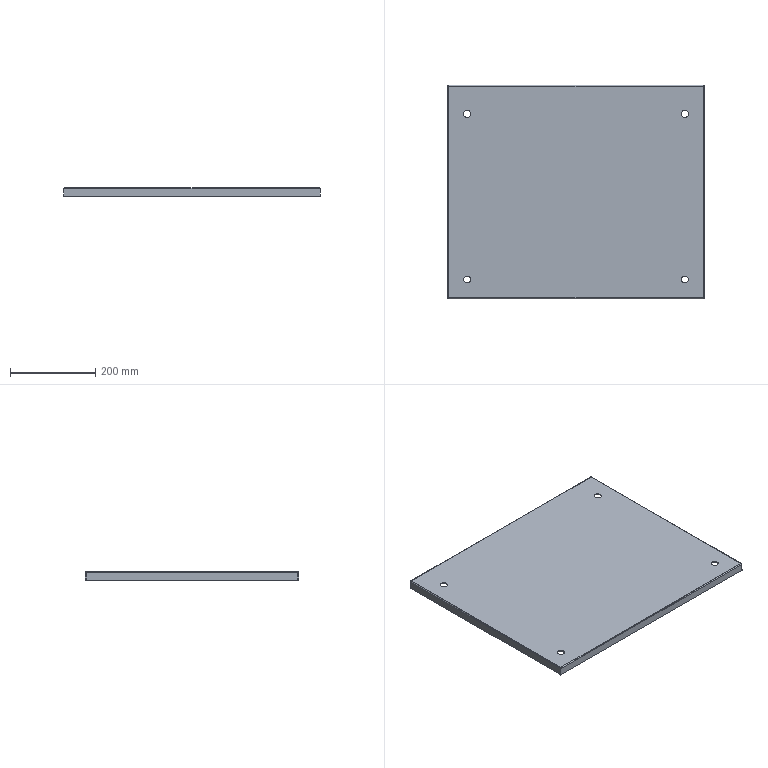Part | SolidWorks | features BaseBody 1, MoveFace 1 | 1 solid | 46 faces | box 600 x 500 x 20 mm | volume 675087 mm3 | plane 30 | cylinder 16 | commonest cylinder face diameters 0.2 x4 4.2 x4 16 x4 17 x4
STEP:
#1=CARTESIAN_POINT('',(187.,-205.,-2.));
#2=VERTEX_POINT('',#1);
#3=CARTESIAN_POINT('',(203.,-205.,-2.));
#4=VERTEX_POINT('',#3);
#5=CARTESIAN_POINT('',(195.,-205.,-2.));
#6=DIRECTION('',(0.,0.,1.));
#7=DIRECTION('',(1.,0.,0.));
#8=AXIS2_PLACEMENT_3D('',#5,#6,#7);
#9=CIRCLE('',#8,8.);
#10=EDGE_CURVE('',#2,#4,#9,.T.);
#11=ORIENTED_EDGE('',*,*,#10,.F.);
#12=CARTESIAN_POINT('',(187.,-205.,0.));
#13=VERTEX_POINT('',#12);
#14=CARTESIAN_POINT('',(187.,-205.,-10.));
#15=DIRECTION('',(0.,0.,1.));
#16=VECTOR('',#15,1000.);
#17=LINE('',#14,#16);
#18=EDGE_CURVE('',#2,#13,#17,.T.);
#19=ORIENTED_EDGE('',*,*,#18,.T.);
#20=CARTESIAN_POINT('',(203.,-205.,0.));
#21=VERTEX_POINT('',#20);
#22=CARTESIAN_POINT('',(195.,-205.,0.));
#23=DIRECTION('',(0.,0.,-1.));
#24=DIRECTION('',(1.,0.,0.));
#25=AXIS2_PLACEMENT_3D('',#22,#23,#24);
#26=CIRCLE('',#25,8.);
#27=EDGE_CURVE('',#21,#13,#26,.T.);
#28=ORIENTED_EDGE('',*,*,#27,.F.);
#29=CARTESIAN_POINT('',(203.,-205.,-10.));
#30=DIRECTION('',(0.,0.,1.));
#31=VECTOR('',#30,1000.);
#32=LINE('',#29,#31);
#33=EDGE_CURVE('',#4,#21,#32,.T.);
#34=ORIENTED_EDGE('',*,*,#33,.F.);
#35=EDGE_LOOP('',(#11,#19,#28,#34));
#36=FACE_OUTER_BOUND('',#35,.T.);
#37=CARTESIAN_POINT('',(195.,-205.,-10.));
#38=DIRECTION('',(0.,0.,1.));
#39=DIRECTION('',(1.,0.,0.));
#40=AXIS2_PLACEMENT_3D('',#37,#38,#39);
#41=CYLINDRICAL_SURFACE('',#40,8.);
#42=ADVANCED_FACE('',(#36),#41,.F.);
#43=CARTESIAN_POINT('',(-323.,-205.,-2.));
#44=VERTEX_POINT('',#43);
#45=CARTESIAN_POINT('',(-307.,-205.,-2.));
#46=VERTEX_POINT('',#45);
#47=CARTESIAN_POINT('',(-315.,-205.,-2.));
#48=DIRECTION('',(0.,0.,1.));
#49=DIRECTION('',(1.,0.,0.));
#50=AXIS2_PLACEMENT_3D('',#47,#48,#49);
#51=CIRCLE('',#50,8.);
#52=EDGE_CURVE('',#44,#46,#51,.T.);
#53=ORIENTED_EDGE('',*,*,#52,.F.);
#54=CARTESIAN_POINT('',(-323.,-205.,0.));
#55=VERTEX_POINT('',#54);
#56=CARTESIAN_POINT('',(-323.,-205.,-10.));
#57=DIRECTION('',(0.,0.,1.));
#58=VECTOR('',#57,1000.);
#59=LINE('',#56,#58);
#60=EDGE_CURVE('',#44,#55,#59,.T.);
#61=ORIENTED_EDGE('',*,*,#60,.T.);
#62=CARTESIAN_POINT('',(-307.,-205.,0.));
#63=VERTEX_POINT('',#62);
#64=CARTESIAN_POINT('',(-315.,-205.,0.));
#65=DIRECTION('',(0.,0.,-1.));
#66=DIRECTION('',(1.,0.,0.));
#67=AXIS2_PLACEMENT_3D('',#64,#65,#66);
#68=CIRCLE('',#67,8.);
#69=EDGE_CURVE('',#63,#55,#68,.T.);
#70=ORIENTED_EDGE('',*,*,#69,.F.);
#71=CARTESIAN_POINT('',(-307.,-205.,-10.));
#72=DIRECTION('',(0.,0.,1.));
#73=VECTOR('',#72,1000.);
#74=LINE('',#71,#73);
#75=EDGE_CURVE('',#46,#63,#74,.T.);
#76=ORIENTED_EDGE('',*,*,#75,.F.);
#77=EDGE_LOOP('',(#53,#61,#70,#76));
#78=FACE_OUTER_BOUND('',#77,.T.);
#79=CARTESIAN_POINT('',(-315.,-205.,-10.));
#80=DIRECTION('',(0.,0.,1.));
#81=DIRECTION('',(1.,0.,0.));
#82=AXIS2_PLACEMENT_3D('',#79,#80,#81);
#83=CYLINDRICAL_SURFACE('',#82,8.);
#84=ADVANCED_FACE('',(#78),#83,.F.);
#85=CARTESIAN_POINT('',(-323.5,183.,-2.));
#86=VERTEX_POINT('',#85);
#87=CARTESIAN_POINT('',(-306.5,183.,-2.));
#88=VERTEX_POINT('',#87);
#89=CARTESIAN_POINT('',(-315.,183.,-2.));
#90=DIRECTION('',(0.,0.,1.));
#91=DIRECTION('',(1.,0.,0.));
#92=AXIS2_PLACEMENT_3D('',#89,#90,#91);
#93=CIRCLE('',#92,8.5);
#94=EDGE_CURVE('',#86,#88,#93,.T.);
#95=ORIENTED_EDGE('',*,*,#94,.F.);
#96=CARTESIAN_POINT('',(-323.5,183.,0.));
#97=VERTEX_POINT('',#96);
#98=CARTESIAN_POINT('',(-323.5,183.,-10.));
#99=DIRECTION('',(0.,0.,1.));
#100=VECTOR('',#99,1000.);
#101=LINE('',#98,#100);
#102=EDGE_CURVE('',#86,#97,#101,.T.);
#103=ORIENTED_EDGE('',*,*,#102,.T.);
#104=CARTESIAN_POINT('',(-306.5,183.,0.));
#105=VERTEX_POINT('',#104);
#106=CARTESIAN_POINT('',(-315.,183.,0.));
#107=DIRECTION('',(0.,0.,-1.));
#108=DIRECTION('',(1.,0.,0.));
#109=AXIS2_PLACEMENT_3D('',#106,#107,#108);
#110=CIRCLE('',#109,8.5);
#111=EDGE_CURVE('',#105,#97,#110,.T.);
#112=ORIENTED_EDGE('',*,*,#111,.F.);
#113=CARTESIAN_POINT('',(-306.5,183.,-10.));
#114=DIRECTION('',(0.,0.,1.));
#115=VECTOR('',#114,1000.);
#116=LINE('',#113,#115);
#117=EDGE_CURVE('',#88,#105,#116,.T.);
#118=ORIENTED_EDGE('',*,*,#117,.F.);
#119=EDGE_LOOP('',(#95,#103,#112,#118));
#120=FACE_OUTER_BOUND('',#119,.T.);
#121=CARTESIAN_POINT('',(-315.,183.,-10.));
#122=DIRECTION('',(0.,0.,1.));
#123=DIRECTION('',(1.,0.,0.));
#124=AXIS2_PLACEMENT_3D('',#121,#122,#123);
#125=CYLINDRICAL_SURFACE('',#124,8.5);
#126=ADVANCED_FACE('',(#120),#125,.F.);
#127=CARTESIAN_POINT('',(186.5,183.,-2.));
#128=VERTEX_POINT('',#127);
#129=CARTESIAN_POINT('',(203.5,183.,-2.));
#130=VERTEX_POINT('',#129);
#131=CARTESIAN_POINT('',(195.,183.,-2.));
#132=DIRECTION('',(0.,0.,1.));
#133=DIRECTION('',(1.,0.,0.));
#134=AXIS2_PLACEMENT_3D('',#131,#132,#133);
#135=CIRCLE('',#134,8.5);
#136=EDGE_CURVE('',#128,#130,#135,.T.);
#137=ORIENTED_EDGE('',*,*,#136,.F.);
#138=CARTESIAN_POINT('',(186.5,183.,0.));
#139=VERTEX_POINT('',#138);
#140=CARTESIAN_POINT('',(186.5,183.,-10.));
#141=DIRECTION('',(0.,0.,1.));
#142=VECTOR('',#141,1000.);
#143=LINE('',#140,#142);
#144=EDGE_CURVE('',#128,#139,#143,.T.);
#145=ORIENTED_EDGE('',*,*,#144,.T.);
#146=CARTESIAN_POINT('',(203.5,183.,0.));
#147=VERTEX_POINT('',#146);
#148=CARTESIAN_POINT('',(195.,183.,0.));
#149=DIRECTION('',(0.,0.,-1.));
#150=DIRECTION('',(1.,0.,0.));
#151=AXIS2_PLACEMENT_3D('',#148,#149,#150);
#152=CIRCLE('',#151,8.5);
#153=EDGE_CURVE('',#147,#139,#152,.T.);
#154=ORIENTED_EDGE('',*,*,#153,.F.);
#155=CARTESIAN_POINT('',(203.5,183.,-10.));
#156=DIRECTION('',(0.,0.,1.));
#157=VECTOR('',#156,1000.);
#158=LINE('',#155,#157);
#159=EDGE_CURVE('',#130,#147,#158,.T.);
#160=ORIENTED_EDGE('',*,*,#159,.F.);
#161=EDGE_LOOP('',(#137,#145,#154,#160));
#162=FACE_OUTER_BOUND('',#161,.T.);
#163=CARTESIAN_POINT('',(195.,183.,-10.));
#164=DIRECTION('',(0.,0.,1.));
#165=DIRECTION('',(1.,0.,0.));
#166=AXIS2_PLACEMENT_3D('',#163,#164,#165);
#167=CYLINDRICAL_SURFACE('',#166,8.5);
#168=ADVANCED_FACE('',(#162),#167,.F.);
#169=CARTESIAN_POINT('',(237.9,247.9,0.));
#170=VERTEX_POINT('',#169);
#171=CARTESIAN_POINT('',(-357.9,247.9,0.));
#172=VERTEX_POINT('',#171);
#173=CARTESIAN_POINT('',(0.,247.9,0.));
#174=DIRECTION('',(-1.,0.,0.));
#175=VECTOR('',#174,1000.);
#176=LINE('',#173,#175);
#177=EDGE_CURVE('',#170,#172,#176,.T.);
#178=ORIENTED_EDGE('',*,*,#177,.T.);
#179=CARTESIAN_POINT('',(-357.9,-247.9,0.));
#180=VERTEX_POINT('',#179);
#181=CARTESIAN_POINT('',(-357.9,0.,0.));
#182=DIRECTION('',(0.,-1.,0.));
#183=VECTOR('',#182,1000.);
#184=LINE('',#181,#183);
#185=EDGE_CURVE('',#172,#180,#184,.T.);
#186=ORIENTED_EDGE('',*,*,#185,.T.);
#187=CARTESIAN_POINT('',(237.9,-247.9,0.));
#188=VERTEX_POINT('',#187);
#189=CARTESIAN_POINT('',(0.,-247.9,0.));
#190=DIRECTION('',(1.,0.,0.));
#191=VECTOR('',#190,1000.);
#192=LINE('',#189,#191);
#193=EDGE_CURVE('',#180,#188,#192,.T.);
#194=ORIENTED_EDGE('',*,*,#193,.T.);
#195=CARTESIAN_POINT('',(237.9,0.,0.));
#196=DIRECTION('',(0.,1.,0.));
#197=VECTOR('',#196,1000.);
#198=LINE('',#195,#197);
#199=EDGE_CURVE('',#188,#170,#198,.T.);
#200=ORIENTED_EDGE('',*,*,#199,.T.);
#201=EDGE_LOOP('',(#178,#186,#194,#200));
#202=FACE_OUTER_BOUND('',#201,.T.);
#203=ORIENTED_EDGE('',*,*,#27,.T.);
#204=CARTESIAN_POINT('',(195.,-205.,0.));
#205=DIRECTION('',(0.,0.,-1.));
#206=DIRECTION('',(1.,0.,0.));
#207=AXIS2_PLACEMENT_3D('',#204,#205,#206);
#208=CIRCLE('',#207,8.);
#209=EDGE_CURVE('',#13,#21,#208,.T.);
#210=ORIENTED_EDGE('',*,*,#209,.T.);
#211=EDGE_LOOP('',(#203,#210));
#212=FACE_BOUND('',#211,.T.);
#213=ORIENTED_EDGE('',*,*,#69,.T.);
#214=CARTESIAN_POINT('',(-315.,-205.,0.));
#215=DIRECTION('',(0.,0.,-1.));
#216=DIRECTION('',(1.,0.,0.));
#217=AXIS2_PLACEMENT_3D('',#214,#215,#216);
#218=CIRCLE('',#217,8.);
#219=EDGE_CURVE('',#55,#63,#218,.T.);
#220=ORIENTED_EDGE('',*,*,#219,.T.);
#221=EDGE_LOOP('',(#213,#220));
#222=FACE_BOUND('',#221,.T.);
#223=ORIENTED_EDGE('',*,*,#111,.T.);
#224=CARTESIAN_POINT('',(-315.,183.,0.));
#225=DIRECTION('',(0.,0.,-1.));
#226=DIRECTION('',(1.,0.,0.));
#227=AXIS2_PLACEMENT_3D('',#224,#225,#226);
#228=CIRCLE('',#227,8.5);
#229=EDGE_CURVE('',#97,#105,#228,.T.);
#230=ORIENTED_EDGE('',*,*,#229,.T.);
#231=EDGE_LOOP('',(#223,#230));
#232=FACE_BOUND('',#231,.T.);
#233=ORIENTED_EDGE('',*,*,#153,.T.);
#234=CARTESIAN_POINT('',(195.,183.,0.));
#235=DIRECTION('',(0.,0.,-1.));
#236=DIRECTION('',(1.,0.,0.));
#237=AXIS2_PLACEMENT_3D('',#234,#235,#236);
#238=CIRCLE('',#237,8.5);
#239=EDGE_CURVE('',#139,#147,#238,.T.);
#240=ORIENTED_EDGE('',*,*,#239,.T.);
#241=EDGE_LOOP('',(#233,#240));
#242=FACE_BOUND('',#241,.T.);
#243=CARTESIAN_POINT('',(0.,0.,0.));
#244=DIRECTION('',(0.,0.,1.));
#245=DIRECTION('',(1.,0.,0.));
#246=AXIS2_PLACEMENT_3D('',#243,#244,#245);
#247=PLANE('',#246);
#248=ADVANCED_FACE('',(#202,#212,#222,#232,#242),#247,.T.);
#249=CARTESIAN_POINT('',(-360.,247.9,-2.1));
#250=VERTEX_POINT('',#249);
#251=CARTESIAN_POINT('',(-360.,-247.9,-2.1));
#252=VERTEX_POINT('',#251);
#253=CARTESIAN_POINT('',(-360.,247.9,-2.1));
#254=DIRECTION('',(0.,-1.,0.));
#255=VECTOR('',#254,1000.);
#256=LINE('',#253,#255);
#257=EDGE_CURVE('',#250,#252,#256,.T.);
#258=ORIENTED_EDGE('',*,*,#257,.T.);
#259=CARTESIAN_POINT('',(-357.9,-247.9,-2.1));
#260=DIRECTION('',(0.,1.,0.));
#261=DIRECTION('',(0.,0.,1.));
#262=AXIS2_PLACEMENT_3D('',#259,#260,#261);
#263=CIRCLE('',#262,2.1);
#264=EDGE_CURVE('',#252,#180,#263,.T.);
#265=ORIENTED_EDGE('',*,*,#264,.T.);
#266=ORIENTED_EDGE('',*,*,#185,.F.);
#267=CARTESIAN_POINT('',(-357.9,247.9,-2.1));
#268=DIRECTION('',(0.,-1.,0.));
#269=DIRECTION('',(0.,0.,1.));
#270=AXIS2_PLACEMENT_3D('',#267,#268,#269);
#271=CIRCLE('',#270,2.1);
#272=EDGE_CURVE('',#172,#250,#271,.T.);
#273=ORIENTED_EDGE('',*,*,#272,.T.);
#274=EDGE_LOOP('',(#258,#265,#266,#273));
#275=FACE_OUTER_BOUND('',#274,.T.);
#276=CARTESIAN_POINT('',(-357.9,247.9,-2.1));
#277=DIRECTION('',(0.,1.,0.));
#278=DIRECTION('',(0.,0.,1.));
#279=AXIS2_PLACEMENT_3D('',#276,#277,#278);
#280=CYLINDRICAL_SURFACE('',#279,2.1);
#281=ADVANCED_FACE('',(#275),#280,.T.);
#282=CARTESIAN_POINT('',(237.9,250.,-2.1));
#283=VERTEX_POINT('',#282);
#284=CARTESIAN_POINT('',(-357.9,250.,-2.1));
#285=VERTEX_POINT('',#284);
#286=CARTESIAN_POINT('',(360.,250.,-2.1));
#287=DIRECTION('',(-1.,0.,0.));
#288=VECTOR('',#287,1000.);
#289=LINE('',#286,#288);
#290=EDGE_CURVE('',#283,#285,#289,.T.);
#291=ORIENTED_EDGE('',*,*,#290,.T.);
#292=CARTESIAN_POINT('',(-357.9,247.9,-2.1));
#293=DIRECTION('',(1.,0.,0.));
#294=DIRECTION('',(0.,0.,-1.));
#295=AXIS2_PLACEMENT_3D('',#292,#293,#294);
#296=CIRCLE('',#295,2.1);
#297=EDGE_CURVE('',#285,#172,#296,.T.);
#298=ORIENTED_EDGE('',*,*,#297,.T.);
#299=ORIENTED_EDGE('',*,*,#177,.F.);
#300=CARTESIAN_POINT('',(237.9,247.9,-2.1));
#301=DIRECTION('',(-1.,0.,0.));
#302=DIRECTION('',(0.,0.,-1.));
#303=AXIS2_PLACEMENT_3D('',#300,#301,#302);
#304=CIRCLE('',#303,2.1);
#305=EDGE_CURVE('',#170,#283,#304,.T.);
#306=ORIENTED_EDGE('',*,*,#305,.T.);
#307=EDGE_LOOP('',(#291,#298,#299,#306));
#308=FACE_OUTER_BOUND('',#307,.T.);
#309=CARTESIAN_POINT('',(360.,247.9,-2.1));
#310=DIRECTION('',(1.,0.,0.));
#311=DIRECTION('',(0.,0.,-1.));
#312=AXIS2_PLACEMENT_3D('',#309,#310,#311);
#313=CYLINDRICAL_SURFACE('',#312,2.1);
#314=ADVANCED_FACE('',(#308),#313,.T.);
#315=CARTESIAN_POINT('',(240.,-247.9,-2.1));
#316=VERTEX_POINT('',#315);
#317=CARTESIAN_POINT('',(240.,247.9,-2.1));
#318=VERTEX_POINT('',#317);
#319=CARTESIAN_POINT('',(240.,-247.9,-2.1));
#320=DIRECTION('',(0.,1.,0.));
#321=VECTOR('',#320,1000.);
#322=LINE('',#319,#321);
#323=EDGE_CURVE('',#316,#318,#322,.T.);
#324=ORIENTED_EDGE('',*,*,#323,.T.);
#325=CARTESIAN_POINT('',(237.9,247.9,-2.1));
#326=DIRECTION('',(0.,-1.,0.));
#327=DIRECTION('',(0.,0.,-1.));
#328=AXIS2_PLACEMENT_3D('',#325,#326,#327);
#329=CIRCLE('',#328,2.1);
#330=EDGE_CURVE('',#318,#170,#329,.T.);
#331=ORIENTED_EDGE('',*,*,#330,.T.);
#332=ORIENTED_EDGE('',*,*,#199,.F.);
#333=CARTESIAN_POINT('',(237.9,-247.9,-2.1));
#334=DIRECTION('',(0.,1.,0.));
#335=DIRECTION('',(0.,0.,-1.));
#336=AXIS2_PLACEMENT_3D('',#333,#334,#335);
#337=CIRCLE('',#336,2.1);
#338=EDGE_CURVE('',#188,#316,#337,.T.);
#339=ORIENTED_EDGE('',*,*,#338,.T.);
#340=EDGE_LOOP('',(#324,#331,#332,#339));
#341=FACE_OUTER_BOUND('',#340,.T.);
#342=CARTESIAN_POINT('',(237.9,-247.9,-2.1));
#343=DIRECTION('',(0.,-1.,0.));
#344=DIRECTION('',(0.,0.,-1.));
#345=AXIS2_PLACEMENT_3D('',#342,#343,#344);
#346=CYLINDRICAL_SURFACE('',#345,2.1);
#347=ADVANCED_FACE('',(#341),#346,.T.);
#348=ORIENTED_EDGE('',*,*,#193,.F.);
#349=CARTESIAN_POINT('',(-357.9,-250.,-2.1));
#350=VERTEX_POINT('',#349);
#351=CARTESIAN_POINT('',(-357.9,-247.9,-2.1));
#352=DIRECTION('',(1.,0.,0.));
#353=DIRECTION('',(0.,0.,1.));
#354=AXIS2_PLACEMENT_3D('',#351,#352,#353);
#355=CIRCLE('',#354,2.1);
#356=EDGE_CURVE('',#180,#350,#355,.T.);
#357=ORIENTED_EDGE('',*,*,#356,.T.);
#358=CARTESIAN_POINT('',(237.9,-250.,-2.1));
#359=VERTEX_POINT('',#358);
#360=CARTESIAN_POINT('',(-360.,-250.,-2.1));
#361=DIRECTION('',(1.,0.,0.));
#362=VECTOR('',#361,1000.);
#363=LINE('',#360,#362);
#364=EDGE_CURVE('',#350,#359,#363,.T.);
#365=ORIENTED_EDGE('',*,*,#364,.T.);
#366=CARTESIAN_POINT('',(237.9,-247.9,-2.1));
#367=DIRECTION('',(-1.,0.,0.));
#368=DIRECTION('',(0.,0.,1.));
#369=AXIS2_PLACEMENT_3D('',#366,#367,#368);
#370=CIRCLE('',#369,2.1);
#371=EDGE_CURVE('',#359,#188,#370,.T.);
#372=ORIENTED_EDGE('',*,*,#371,.T.);
#373=EDGE_LOOP('',(#348,#357,#365,#372));
#374=FACE_OUTER_BOUND('',#373,.T.);
#375=CARTESIAN_POINT('',(-360.,-247.9,-2.1));
#376=DIRECTION('',(-1.,0.,0.));
#377=DIRECTION('',(0.,0.,1.));
#378=AXIS2_PLACEMENT_3D('',#375,#376,#377);
#379=CYLINDRICAL_SURFACE('',#378,2.1);
#380=ADVANCED_FACE('',(#374),#379,.T.);
#381=ORIENTED_EDGE('',*,*,#18,.F.);
#382=CARTESIAN_POINT('',(195.,-205.,-2.));
#383=DIRECTION('',(0.,0.,1.));
#384=DIRECTION('',(1.,0.,0.));
#385=AXIS2_PLACEMENT_3D('',#382,#383,#384);
#386=CIRCLE('',#385,8.);
#387=EDGE_CURVE('',#4,#2,#386,.T.);
#388=ORIENTED_EDGE('',*,*,#387,.F.);
#389=ORIENTED_EDGE('',*,*,#33,.T.);
#390=ORIENTED_EDGE('',*,*,#209,.F.);
#391=EDGE_LOOP('',(#381,#388,#389,#390));
#392=FACE_OUTER_BOUND('',#391,.T.);
#393=CARTESIAN_POINT('',(195.,-205.,-10.));
#394=DIRECTION('',(0.,0.,1.));
#395=DIRECTION('',(1.,0.,0.));
#396=AXIS2_PLACEMENT_3D('',#393,#394,#395);
#397=CYLINDRICAL_SURFACE('',#396,8.);
#398=ADVANCED_FACE('',(#392),#397,.F.);
#399=ORIENTED_EDGE('',*,*,#60,.F.);
#400=CARTESIAN_POINT('',(-315.,-205.,-2.));
#401=DIRECTION('',(0.,0.,1.));
#402=DIRECTION('',(1.,0.,0.));
#403=AXIS2_PLACEMENT_3D('',#400,#401,#402);
#404=CIRCLE('',#403,8.);
#405=EDGE_CURVE('',#46,#44,#404,.T.);
#406=ORIENTED_EDGE('',*,*,#405,.F.);
#407=ORIENTED_EDGE('',*,*,#75,.T.);
#408=ORIENTED_EDGE('',*,*,#219,.F.);
#409=EDGE_LOOP('',(#399,#406,#407,#408));
#410=FACE_OUTER_BOUND('',#409,.T.);
#411=CARTESIAN_POINT('',(-315.,-205.,-10.));
#412=DIRECTION('',(0.,0.,1.));
#413=DIRECTION('',(1.,0.,0.));
#414=AXIS2_PLACEMENT_3D('',#411,#412,#413);
#415=CYLINDRICAL_SURFACE('',#414,8.);
#416=ADVANCED_FACE('',(#410),#415,.F.);
#417=ORIENTED_EDGE('',*,*,#102,.F.);
#418=CARTESIAN_POINT('',(-315.,183.,-2.));
#419=DIRECTION('',(0.,0.,1.));
#420=DIRECTION('',(1.,0.,0.));
#421=AXIS2_PLACEMENT_3D('',#418,#419,#420);
#422=CIRCLE('',#421,8.5);
#423=EDGE_CURVE('',#88,#86,#422,.T.);
#424=ORIENTED_EDGE('',*,*,#423,.F.);
#425=ORIENTED_EDGE('',*,*,#117,.T.);
#426=ORIENTED_EDGE('',*,*,#229,.F.);
#427=EDGE_LOOP('',(#417,#424,#425,#426));
#428=FACE_OUTER_BOUND('',#427,.T.);
#429=CARTESIAN_POINT('',(-315.,183.,-10.));
#430=DIRECTION('',(0.,0.,1.));
#431=DIRECTION('',(1.,0.,0.));
#432=AXIS2_PLACEMENT_3D('',#429,#430,#431);
#433=CYLINDRICAL_SURFACE('',#432,8.5);
#434=ADVANCED_FACE('',(#428),#433,.F.);
#435=ORIENTED_EDGE('',*,*,#144,.F.);
#436=CARTESIAN_POINT('',(195.,183.,-2.));
#437=DIRECTION('',(0.,0.,1.));
#438=DIRECTION('',(1.,0.,0.));
#439=AXIS2_PLACEMENT_3D('',#436,#437,#438);
#440=CIRCLE('',#439,8.5);
#441=EDGE_CURVE('',#130,#128,#440,.T.);
#442=ORIENTED_EDGE('',*,*,#441,.F.);
#443=ORIENTED_EDGE('',*,*,#159,.T.);
#444=ORIENTED_EDGE('',*,*,#239,.F.);
#445=EDGE_LOOP('',(#435,#442,#443,#444));
#446=FACE_OUTER_BOUND('',#445,.T.);
#447=CARTESIAN_POINT('',(195.,183.,-10.));
#448=DIRECTION('',(0.,0.,1.));
#449=DIRECTION('',(1.,0.,0.));
#450=AXIS2_PLACEMENT_3D('',#447,#448,#449);
#451=CYLINDRICAL_SURFACE('',#450,8.5);
#452=ADVANCED_FACE('',(#446),#451,.F.);
#453=CARTESIAN_POINT('',(-357.9,-247.9,-2.));
#454=VERTEX_POINT('',#453);
#455=CARTESIAN_POINT('',(-357.9,-247.9,-2.1));
#456=DIRECTION('',(0.,0.,1.));
#457=VECTOR('',#456,1000.);
#458=LINE('',#455,#457);
#459=EDGE_CURVE('',#454,#180,#458,.T.);
#460=ORIENTED_EDGE('',*,*,#459,.T.);
#461=ORIENTED_EDGE('',*,*,#264,.F.);
#462=CARTESIAN_POINT('',(-360.,-247.9,-20.));
#463=VERTEX_POINT('',#462);
#464=CARTESIAN_POINT('',(-360.,-247.9,0.));
#465=DIRECTION('',(0.,0.,-1.));
#466=VECTOR('',#465,1000.);
#467=LINE('',#464,#466);
#468=EDGE_CURVE('',#252,#463,#467,.T.);
#469=ORIENTED_EDGE('',*,*,#468,.T.);
#470=CARTESIAN_POINT('',(-358.,-247.9,-20.));
#471=VERTEX_POINT('',#470);
#472=CARTESIAN_POINT('',(-360.,-247.9,-20.));
#473=DIRECTION('',(-1.,0.,0.));
#474=VECTOR('',#473,1000.);
#475=LINE('',#472,#474);
#476=EDGE_CURVE('',#471,#463,#475,.T.);
#477=ORIENTED_EDGE('',*,*,#476,.F.);
#478=CARTESIAN_POINT('',(-358.,-247.9,-2.1));
#479=VERTEX_POINT('',#478);
#480=CARTESIAN_POINT('',(-358.,-247.9,-2.));
#481=DIRECTION('',(0.,0.,-1.));
#482=VECTOR('',#481,1000.);
#483=LINE('',#480,#482);
#484=EDGE_CURVE('',#479,#471,#483,.T.);
#485=ORIENTED_EDGE('',*,*,#484,.F.);
#486=CARTESIAN_POINT('',(-357.9,-247.9,-2.1));
#487=DIRECTION('',(0.,1.,0.));
#488=DIRECTION('',(0.,0.,1.));
#489=AXIS2_PLACEMENT_3D('',#486,#487,#488);
#490=CIRCLE('',#489,0.1);
#491=EDGE_CURVE('',#479,#454,#490,.T.);
#492=ORIENTED_EDGE('',*,*,#491,.T.);
#493=EDGE_LOOP('',(#460,#461,#469,#477,#485,#492));
#494=FACE_OUTER_BOUND('',#493,.T.);
#495=CARTESIAN_POINT('',(-357.9,-247.9,-2.1));
#496=DIRECTION('',(0.,-1.,0.));
#497=DIRECTION('',(0.,0.,-1.));
#498=AXIS2_PLACEMENT_3D('',#495,#496,#497);
#499=PLANE('',#498);
#500=ADVANCED_FACE('',(#494),#499,.T.);
#501=CARTESIAN_POINT('',(-360.,247.9,-20.));
#502=VERTEX_POINT('',#501);
#503=CARTESIAN_POINT('',(-360.,247.9,0.));
#504=DIRECTION('',(0.,0.,1.));
#505=VECTOR('',#504,1000.);
#506=LINE('',#503,#505);
#507=EDGE_CURVE('',#502,#250,#506,.T.);
#508=ORIENTED_EDGE('',*,*,#507,.F.);
#509=CARTESIAN_POINT('',(-360.,0.,-20.));
#510=DIRECTION('',(0.,1.,0.));
#511=VECTOR('',#510,1000.);
#512=LINE('',#509,#511);
#513=EDGE_CURVE('',#463,#502,#512,.T.);
#514=ORIENTED_EDGE('',*,*,#513,.F.);
#515=ORIENTED_EDGE('',*,*,#468,.F.);
#516=ORIENTED_EDGE('',*,*,#257,.F.);
#517=EDGE_LOOP('',(#508,#514,#515,#516));
#518=FACE_OUTER_BOUND('',#517,.T.);
#519=CARTESIAN_POINT('',(-360.,0.,0.));
#520=DIRECTION('',(1.,0.,0.));
#521=DIRECTION('',(0.,0.,-1.));
#522=AXIS2_PLACEMENT_3D('',#519,#520,#521);
#523=PLANE('',#522);
#524=ADVANCED_FACE('',(#518),#523,.F.);
#525=CARTESIAN_POINT('',(-357.9,247.9,-2.));
#526=VERTEX_POINT('',#525);
#527=CARTESIAN_POINT('',(-358.,247.9,-2.1));
#528=VERTEX_POINT('',#527);
#529=CARTESIAN_POINT('',(-357.9,247.9,-2.1));
#530=DIRECTION('',(0.,-1.,0.));
#531=DIRECTION('',(0.,0.,1.));
#532=AXIS2_PLACEMENT_3D('',#529,#530,#531);
#533=CIRCLE('',#532,0.1);
#534=EDGE_CURVE('',#526,#528,#533,.T.);
#535=ORIENTED_EDGE('',*,*,#534,.T.);
#536=CARTESIAN_POINT('',(-358.,247.9,-20.));
#537=VERTEX_POINT('',#536);
#538=CARTESIAN_POINT('',(-358.,247.9,-20.));
#539=DIRECTION('',(0.,0.,1.));
#540=VECTOR('',#539,1000.);
#541=LINE('',#538,#540);
#542=EDGE_CURVE('',#537,#528,#541,.T.);
#543=ORIENTED_EDGE('',*,*,#542,.F.);
#544=CARTESIAN_POINT('',(-360.,247.9,-20.));
#545=DIRECTION('',(1.,0.,0.));
#546=VECTOR('',#545,1000.);
#547=LINE('',#544,#546);
#548=EDGE_CURVE('',#502,#537,#547,.T.);
#549=ORIENTED_EDGE('',*,*,#548,.F.);
#550=ORIENTED_EDGE('',*,*,#507,.T.);
#551=ORIENTED_EDGE('',*,*,#272,.F.);
#552=CARTESIAN_POINT('',(-357.9,247.9,-2.1));
#553=DIRECTION('',(0.,0.,1.));
#554=VECTOR('',#553,1000.);
#555=LINE('',#552,#554);
#556=EDGE_CURVE('',#526,#172,#555,.T.);
#557=ORIENTED_EDGE('',*,*,#556,.F.);
#558=EDGE_LOOP('',(#535,#543,#549,#550,#551,#557));
#559=FACE_OUTER_BOUND('',#558,.T.);
#560=CARTESIAN_POINT('',(-357.9,247.9,-2.1));
#561=DIRECTION('',(0.,-1.,0.));
#562=DIRECTION('',(0.,0.,-1.));
#563=AXIS2_PLACEMENT_3D('',#560,#561,#562);
#564=PLANE('',#563);
#565=ADVANCED_FACE('',(#559),#564,.F.);
#566=CARTESIAN_POINT('',(-357.9,248.,-2.1));
#567=VERTEX_POINT('',#566);
#568=CARTESIAN_POINT('',(-357.9,247.9,-2.1));
#569=DIRECTION('',(1.,0.,0.));
#570=DIRECTION('',(0.,0.,-1.));
#571=AXIS2_PLACEMENT_3D('',#568,#569,#570);
#572=CIRCLE('',#571,0.1);
#573=EDGE_CURVE('',#567,#526,#572,.T.);
#574=ORIENTED_EDGE('',*,*,#573,.T.);
#575=ORIENTED_EDGE('',*,*,#556,.T.);
#576=ORIENTED_EDGE('',*,*,#297,.F.);
#577=CARTESIAN_POINT('',(-357.9,247.9,-2.1));
#578=DIRECTION('',(0.,-1.,0.));
#579=VECTOR('',#578,1000.);
#580=LINE('',#577,#579);
#581=EDGE_CURVE('',#285,#567,#580,.T.);
#582=ORIENTED_EDGE('',*,*,#581,.T.);
#583=EDGE_LOOP('',(#574,#575,#576,#582));
#584=FACE_OUTER_BOUND('',#583,.T.);
#585=CARTESIAN_POINT('',(-357.9,247.9,-2.1));
#586=DIRECTION('',(-1.,0.,0.));
#587=DIRECTION('',(0.,0.,1.));
#588=AXIS2_PLACEMENT_3D('',#585,#586,#587);
#589=PLANE('',#588);
#590=ADVANCED_FACE('',(#584),#589,.T.);
#591=CARTESIAN_POINT('',(240.,250.,-20.));
#592=VERTEX_POINT('',#591);
#593=CARTESIAN_POINT('',(240.,250.,-2.1));
#594=VERTEX_POINT('',#593);
#595=CARTESIAN_POINT('',(240.,250.,0.));
#596=DIRECTION('',(0.,0.,1.));
#597=VECTOR('',#596,1000.);
#598=LINE('',#595,#597);
#599=EDGE_CURVE('',#592,#594,#598,.T.);
#600=ORIENTED_EDGE('',*,*,#599,.F.);
#601=CARTESIAN_POINT('',(-360.,250.,-20.));
#602=VERTEX_POINT('',#601);
#603=CARTESIAN_POINT('',(0.,250.,-20.));
#604=DIRECTION('',(1.,0.,0.));
#605=VECTOR('',#604,1000.);
#606=LINE('',#603,#605);
#607=EDGE_CURVE('',#602,#592,#606,.T.);
#608=ORIENTED_EDGE('',*,*,#607,.F.);
#609=CARTESIAN_POINT('',(-360.,250.,-2.1));
#610=VERTEX_POINT('',#609);
#611=CARTESIAN_POINT('',(-360.,250.,0.));
#612=DIRECTION('',(0.,0.,-1.));
#613=VECTOR('',#612,1000.);
#614=LINE('',#611,#613);
#615=EDGE_CURVE('',#610,#602,#614,.T.);
#616=ORIENTED_EDGE('',*,*,#615,.F.);
#617=CARTESIAN_POINT('',(0.,250.,-2.1));
#618=DIRECTION('',(-1.,0.,0.));
#619=VECTOR('',#618,1000.);
#620=LINE('',#617,#619);
#621=EDGE_CURVE('',#285,#610,#620,.T.);
#622=ORIENTED_EDGE('',*,*,#621,.F.);
#623=ORIENTED_EDGE('',*,*,#290,.F.);
#624=CARTESIAN_POINT('',(0.,250.,-2.1));
#625=DIRECTION('',(-1.,0.,0.));
#626=VECTOR('',#625,1000.);
#627=LINE('',#624,#626);
#628=EDGE_CURVE('',#594,#283,#627,.T.);
#629=ORIENTED_EDGE('',*,*,#628,.F.);
#630=EDGE_LOOP('',(#600,#608,#616,#622,#623,#629));
#631=FACE_OUTER_BOUND('',#630,.T.);
#632=CARTESIAN_POINT('',(0.,250.,0.));
#633=DIRECTION('',(0.,-1.,0.));
#634=DIRECTION('',(0.,0.,-1.));
#635=AXIS2_PLACEMENT_3D('',#632,#633,#634);
#636=PLANE('',#635);
#637=ADVANCED_FACE('',(#631),#636,.F.);
#638=ORIENTED_EDGE('',*,*,#305,.F.);
#639=CARTESIAN_POINT('',(237.9,247.9,-2.));
#640=VERTEX_POINT('',#639);
#641=CARTESIAN_POINT('',(237.9,247.9,-2.1));
#642=DIRECTION('',(0.,0.,-1.));
#643=VECTOR('',#642,1000.);
#644=LINE('',#641,#643);
#645=EDGE_CURVE('',#170,#640,#644,.T.);
#646=ORIENTED_EDGE('',*,*,#645,.T.);
#647=CARTESIAN_POINT('',(237.9,248.,-2.1));
#648=VERTEX_POINT('',#647);
#649=CARTESIAN_POINT('',(237.9,247.9,-2.1));
#650=DIRECTION('',(-1.,0.,0.));
#651=DIRECTION('',(0.,0.,-1.));
#652=AXIS2_PLACEMENT_3D('',#649,#650,#651);
#653=CIRCLE('',#652,0.1);
#654=EDGE_CURVE('',#640,#648,#653,.T.);
#655=ORIENTED_EDGE('',*,*,#654,.T.);
#656=CARTESIAN_POINT('',(237.9,247.9,-2.1));
#657=DIRECTION('',(0.,1.,0.));
#658=VECTOR('',#657,1000.);
#659=LINE('',#656,#658);
#660=EDGE_CURVE('',#648,#283,#659,.T.);
#661=ORIENTED_EDGE('',*,*,#660,.T.);
#662=EDGE_LOOP('',(#638,#646,#655,#661));
#663=FACE_OUTER_BOUND('',#662,.T.);
#664=CARTESIAN_POINT('',(237.9,247.9,-2.1));
#665=DIRECTION('',(1.,0.,0.));
#666=DIRECTION('',(0.,0.,-1.));
#667=AXIS2_PLACEMENT_3D('',#664,#665,#666);
#668=PLANE('',#667);
#669=ADVANCED_FACE('',(#663),#668,.T.);
#670=ORIENTED_EDGE('',*,*,#645,.F.);
#671=ORIENTED_EDGE('',*,*,#330,.F.);
#672=CARTESIAN_POINT('',(240.,247.9,-20.));
#673=VERTEX_POINT('',#672);
#674=CARTESIAN_POINT('',(240.,247.9,0.));
#675=DIRECTION('',(0.,0.,-1.));
#676=VECTOR('',#675,1000.);
#677=LINE('',#674,#676);
#678=EDGE_CURVE('',#318,#673,#677,.T.);
#679=ORIENTED_EDGE('',*,*,#678,.T.);
#680=CARTESIAN_POINT('',(238.,247.9,-20.));
#681=VERTEX_POINT('',#680);
#682=CARTESIAN_POINT('',(360.,247.9,-20.));
#683=DIRECTION('',(1.,0.,0.));
#684=VECTOR('',#683,1000.);
#685=LINE('',#682,#684);
#686=EDGE_CURVE('',#681,#673,#685,.T.);
#687=ORIENTED_EDGE('',*,*,#686,.F.);
#688=CARTESIAN_POINT('',(238.,247.9,-2.1));
#689=VERTEX_POINT('',#688);
#690=CARTESIAN_POINT('',(238.,247.9,-2.));
#691=DIRECTION('',(0.,0.,-1.));
#692=VECTOR('',#691,1000.);
#693=LINE('',#690,#692);
#694=EDGE_CURVE('',#689,#681,#693,.T.);
#695=ORIENTED_EDGE('',*,*,#694,.F.);
#696=CARTESIAN_POINT('',(237.9,247.9,-2.1));
#697=DIRECTION('',(0.,-1.,0.));
#698=DIRECTION('',(0.,0.,-1.));
#699=AXIS2_PLACEMENT_3D('',#696,#697,#698);
#700=CIRCLE('',#699,0.1);
#701=EDGE_CURVE('',#689,#640,#700,.T.);
#702=ORIENTED_EDGE('',*,*,#701,.T.);
#703=EDGE_LOOP('',(#670,#671,#679,#687,#695,#702));
#704=FACE_OUTER_BOUND('',#703,.T.);
#705=CARTESIAN_POINT('',(357.9,247.9,-2.1));
#706=DIRECTION('',(0.,1.,0.));
#707=DIRECTION('',(0.,0.,1.));
#708=AXIS2_PLACEMENT_3D('',#705,#706,#707);
#709=PLANE('',#708);
#710=ADVANCED_FACE('',(#704),#709,.T.);
#711=CARTESIAN_POINT('',(240.,-247.9,-20.));
#712=VERTEX_POINT('',#711);
#713=CARTESIAN_POINT('',(240.,-247.9,0.));
#714=DIRECTION('',(0.,0.,1.));
#715=VECTOR('',#714,1000.);
#716=LINE('',#713,#715);
#717=EDGE_CURVE('',#712,#316,#716,.T.);
#718=ORIENTED_EDGE('',*,*,#717,.F.);
#719=CARTESIAN_POINT('',(240.,0.,-20.));
#720=DIRECTION('',(0.,-1.,0.));
#721=VECTOR('',#720,1000.);
#722=LINE('',#719,#721);
#723=EDGE_CURVE('',#673,#712,#722,.T.);
#724=ORIENTED_EDGE('',*,*,#723,.F.);
#725=ORIENTED_EDGE('',*,*,#678,.F.);
#726=ORIENTED_EDGE('',*,*,#323,.F.);
#727=EDGE_LOOP('',(#718,#724,#725,#726));
#728=FACE_OUTER_BOUND('',#727,.T.);
#729=CARTESIAN_POINT('',(240.,0.,0.));
#730=DIRECTION('',(-1.,0.,0.));
#731=DIRECTION('',(0.,0.,1.));
#732=AXIS2_PLACEMENT_3D('',#729,#730,#731);
#733=PLANE('',#732);
#734=ADVANCED_FACE('',(#728),#733,.F.);
#735=CARTESIAN_POINT('',(237.9,-247.9,-2.));
#736=VERTEX_POINT('',#735);
#737=CARTESIAN_POINT('',(238.,-247.9,-2.1));
#738=VERTEX_POINT('',#737);
#739=CARTESIAN_POINT('',(237.9,-247.9,-2.1));
#740=DIRECTION('',(0.,1.,0.));
#741=DIRECTION('',(0.,0.,-1.));
#742=AXIS2_PLACEMENT_3D('',#739,#740,#741);
#743=CIRCLE('',#742,0.1);
#744=EDGE_CURVE('',#736,#738,#743,.T.);
#745=ORIENTED_EDGE('',*,*,#744,.T.);
#746=CARTESIAN_POINT('',(238.,-247.9,-20.));
#747=VERTEX_POINT('',#746);
#748=CARTESIAN_POINT('',(238.,-247.9,-20.));
#749=DIRECTION('',(0.,0.,1.));
#750=VECTOR('',#749,1000.);
#751=LINE('',#748,#750);
#752=EDGE_CURVE('',#747,#738,#751,.T.);
#753=ORIENTED_EDGE('',*,*,#752,.F.);
#754=CARTESIAN_POINT('',(360.,-247.9,-20.));
#755=DIRECTION('',(-1.,0.,0.));
#756=VECTOR('',#755,1000.);
#757=LINE('',#754,#756);
#758=EDGE_CURVE('',#712,#747,#757,.T.);
#759=ORIENTED_EDGE('',*,*,#758,.F.);
#760=ORIENTED_EDGE('',*,*,#717,.T.);
#761=ORIENTED_EDGE('',*,*,#338,.F.);
#762=CARTESIAN_POINT('',(237.9,-247.9,-2.1));
#763=DIRECTION('',(0.,0.,1.));
#764=VECTOR('',#763,1000.);
#765=LINE('',#762,#764);
#766=EDGE_CURVE('',#736,#188,#765,.T.);
#767=ORIENTED_EDGE('',*,*,#766,.F.);
#768=EDGE_LOOP('',(#745,#753,#759,#760,#761,#767));
#769=FACE_OUTER_BOUND('',#768,.T.);
#770=CARTESIAN_POINT('',(357.9,-247.9,-2.1));
#771=DIRECTION('',(0.,1.,0.));
#772=DIRECTION('',(0.,0.,1.));
#773=AXIS2_PLACEMENT_3D('',#770,#771,#772);
#774=PLANE('',#773);
#775=ADVANCED_FACE('',(#769),#774,.F.);
#776=ORIENTED_EDGE('',*,*,#356,.F.);
#777=ORIENTED_EDGE('',*,*,#459,.F.);
#778=CARTESIAN_POINT('',(-357.9,-248.,-2.1));
#779=VERTEX_POINT('',#778);
#780=CARTESIAN_POINT('',(-357.9,-247.9,-2.1));
#781=DIRECTION('',(1.,0.,0.));
#782=DIRECTION('',(0.,0.,1.));
#783=AXIS2_PLACEMENT_3D('',#780,#781,#782);
#784=CIRCLE('',#783,0.1);
#785=EDGE_CURVE('',#454,#779,#784,.T.);
#786=ORIENTED_EDGE('',*,*,#785,.T.);
#787=CARTESIAN_POINT('',(-357.9,-247.9,-2.1));
#788=DIRECTION('',(0.,-1.,0.));
#789=VECTOR('',#788,1000.);
#790=LINE('',#787,#789);
#791=EDGE_CURVE('',#779,#350,#790,.T.);
#792=ORIENTED_EDGE('',*,*,#791,.T.);
#793=EDGE_LOOP('',(#776,#777,#786,#792));
#794=FACE_OUTER_BOUND('',#793,.T.);
#795=CARTESIAN_POINT('',(-357.9,-247.9,-2.1));
#796=DIRECTION('',(-1.,0.,0.));
#797=DIRECTION('',(0.,0.,1.));
#798=AXIS2_PLACEMENT_3D('',#795,#796,#797);
#799=PLANE('',#798);
#800=ADVANCED_FACE('',(#794),#799,.T.);
#801=CARTESIAN_POINT('',(237.9,-248.,-2.1));
#802=VERTEX_POINT('',#801);
#803=CARTESIAN_POINT('',(237.9,-247.9,-2.1));
#804=DIRECTION('',(-1.,0.,0.));
#805=DIRECTION('',(0.,0.,1.));
#806=AXIS2_PLACEMENT_3D('',#803,#804,#805);
#807=CIRCLE('',#806,0.1);
#808=EDGE_CURVE('',#802,#736,#807,.T.);
#809=ORIENTED_EDGE('',*,*,#808,.T.);
#810=ORIENTED_EDGE('',*,*,#766,.T.);
#811=ORIENTED_EDGE('',*,*,#371,.F.);
#812=CARTESIAN_POINT('',(237.9,-247.9,-2.1));
#813=DIRECTION('',(0.,1.,0.));
#814=VECTOR('',#813,1000.);
#815=LINE('',#812,#814);
#816=EDGE_CURVE('',#359,#802,#815,.T.);
#817=ORIENTED_EDGE('',*,*,#816,.T.);
#818=EDGE_LOOP('',(#809,#810,#811,#817));
#819=FACE_OUTER_BOUND('',#818,.T.);
#820=CARTESIAN_POINT('',(237.9,-247.9,-2.1));
#821=DIRECTION('',(1.,0.,0.));
#822=DIRECTION('',(0.,0.,-1.));
#823=AXIS2_PLACEMENT_3D('',#820,#821,#822);
#824=PLANE('',#823);
#825=ADVANCED_FACE('',(#819),#824,.T.);
#826=CARTESIAN_POINT('',(-360.,-250.,-20.));
#827=VERTEX_POINT('',#826);
#828=CARTESIAN_POINT('',(-360.,-250.,-2.1));
#829=VERTEX_POINT('',#828);
#830=CARTESIAN_POINT('',(-360.,-250.,0.));
#831=DIRECTION('',(0.,0.,1.));
#832=VECTOR('',#831,1000.);
#833=LINE('',#830,#832);
#834=EDGE_CURVE('',#827,#829,#833,.T.);
#835=ORIENTED_EDGE('',*,*,#834,.F.);
#836=CARTESIAN_POINT('',(240.,-250.,-20.));
#837=VERTEX_POINT('',#836);
#838=CARTESIAN_POINT('',(0.,-250.,-20.));
#839=DIRECTION('',(-1.,0.,0.));
#840=VECTOR('',#839,1000.);
#841=LINE('',#838,#840);
#842=EDGE_CURVE('',#837,#827,#841,.T.);
#843=ORIENTED_EDGE('',*,*,#842,.F.);
#844=CARTESIAN_POINT('',(240.,-250.,-2.1));
#845=VERTEX_POINT('',#844);
#846=CARTESIAN_POINT('',(240.,-250.,0.));
#847=DIRECTION('',(0.,0.,-1.));
#848=VECTOR('',#847,1000.);
#849=LINE('',#846,#848);
#850=EDGE_CURVE('',#845,#837,#849,.T.);
#851=ORIENTED_EDGE('',*,*,#850,.F.);
#852=CARTESIAN_POINT('',(0.,-250.,-2.1));
#853=DIRECTION('',(1.,0.,0.));
#854=VECTOR('',#853,1000.);
#855=LINE('',#852,#854);
#856=EDGE_CURVE('',#359,#845,#855,.T.);
#857=ORIENTED_EDGE('',*,*,#856,.F.);
#858=ORIENTED_EDGE('',*,*,#364,.F.);
#859=CARTESIAN_POINT('',(0.,-250.,-2.1));
#860=DIRECTION('',(1.,0.,0.));
#861=VECTOR('',#860,1000.);
#862=LINE('',#859,#861);
#863=EDGE_CURVE('',#829,#350,#862,.T.);
#864=ORIENTED_EDGE('',*,*,#863,.F.);
#865=EDGE_LOOP('',(#835,#843,#851,#857,#858,#864));
#866=FACE_OUTER_BOUND('',#865,.T.);
#867=CARTESIAN_POINT('',(0.,-250.,0.));
#868=DIRECTION('',(0.,1.,0.));
#869=DIRECTION('',(0.,0.,1.));
#870=AXIS2_PLACEMENT_3D('',#867,#868,#869);
#871=PLANE('',#870);
#872=ADVANCED_FACE('',(#866),#871,.F.);
#873=CARTESIAN_POINT('',(0.,-247.9,-2.));
#874=DIRECTION('',(1.,0.,0.));
#875=VECTOR('',#874,1000.);
#876=LINE('',#873,#875);
#877=EDGE_CURVE('',#454,#736,#876,.T.);
#878=ORIENTED_EDGE('',*,*,#877,.F.);
#879=CARTESIAN_POINT('',(-357.9,0.,-2.));
#880=DIRECTION('',(0.,-1.,0.));
#881=VECTOR('',#880,1000.);
#882=LINE('',#879,#881);
#883=EDGE_CURVE('',#526,#454,#882,.T.);
#884=ORIENTED_EDGE('',*,*,#883,.F.);
#885=CARTESIAN_POINT('',(0.,247.9,-2.));
#886=DIRECTION('',(-1.,0.,0.));
#887=VECTOR('',#886,1000.);
#888=LINE('',#885,#887);
#889=EDGE_CURVE('',#640,#526,#888,.T.);
#890=ORIENTED_EDGE('',*,*,#889,.F.);
#891=CARTESIAN_POINT('',(237.9,0.,-2.));
#892=DIRECTION('',(0.,1.,0.));
#893=VECTOR('',#892,1000.);
#894=LINE('',#891,#893);
#895=EDGE_CURVE('',#736,#640,#894,.T.);
#896=ORIENTED_EDGE('',*,*,#895,.F.);
#897=EDGE_LOOP('',(#878,#884,#890,#896));
#898=FACE_OUTER_BOUND('',#897,.T.);
#899=ORIENTED_EDGE('',*,*,#387,.T.);
#900=ORIENTED_EDGE('',*,*,#10,.T.);
#901=EDGE_LOOP('',(#899,#900));
#902=FACE_BOUND('',#901,.T.);
#903=ORIENTED_EDGE('',*,*,#405,.T.);
#904=ORIENTED_EDGE('',*,*,#52,.T.);
#905=EDGE_LOOP('',(#903,#904));
#906=FACE_BOUND('',#905,.T.);
#907=ORIENTED_EDGE('',*,*,#423,.T.);
#908=ORIENTED_EDGE('',*,*,#94,.T.);
#909=EDGE_LOOP('',(#907,#908));
#910=FACE_BOUND('',#909,.T.);
#911=ORIENTED_EDGE('',*,*,#441,.T.);
#912=ORIENTED_EDGE('',*,*,#136,.T.);
#913=EDGE_LOOP('',(#911,#912));
#914=FACE_BOUND('',#913,.T.);
#915=CARTESIAN_POINT('',(0.,0.,-2.));
#916=DIRECTION('',(0.,0.,1.));
#917=DIRECTION('',(1.,0.,0.));
#918=AXIS2_PLACEMENT_3D('',#915,#916,#917);
#919=PLANE('',#918);
#920=ADVANCED_FACE('',(#898,#902,#906,#910,#914),#919,.F.);
#921=ORIENTED_EDGE('',*,*,#476,.T.);
#922=ORIENTED_EDGE('',*,*,#513,.T.);
#923=ORIENTED_EDGE('',*,*,#548,.T.);
#924=CARTESIAN_POINT('',(-358.,-247.9,-20.));
#925=DIRECTION('',(0.,1.,0.));
#926=VECTOR('',#925,1000.);
#927=LINE('',#924,#926);
#928=EDGE_CURVE('',#471,#537,#927,.T.);
#929=ORIENTED_EDGE('',*,*,#928,.F.);
#930=EDGE_LOOP('',(#921,#922,#923,#929));
#931=FACE_OUTER_BOUND('',#930,.T.);
#932=CARTESIAN_POINT('',(-360.,-247.9,-20.));
#933=DIRECTION('',(0.,0.,1.));
#934=DIRECTION('',(1.,0.,0.));
#935=AXIS2_PLACEMENT_3D('',#932,#933,#934);
#936=PLANE('',#935);
#937=ADVANCED_FACE('',(#931),#936,.F.);
#938=CARTESIAN_POINT('',(-360.,248.,-2.1));
#939=VERTEX_POINT('',#938);
#940=CARTESIAN_POINT('',(-360.,0.,-2.1));
#941=DIRECTION('',(0.,-1.,0.));
#942=VECTOR('',#941,1000.);
#943=LINE('',#940,#942);
#944=EDGE_CURVE('',#610,#939,#943,.T.);
#945=ORIENTED_EDGE('',*,*,#944,.T.);
#946=CARTESIAN_POINT('',(0.,248.,-2.1));
#947=DIRECTION('',(1.,0.,0.));
#948=VECTOR('',#947,1000.);
#949=LINE('',#946,#948);
#950=EDGE_CURVE('',#939,#567,#949,.T.);
#951=ORIENTED_EDGE('',*,*,#950,.T.);
#952=ORIENTED_EDGE('',*,*,#581,.F.);
#953=ORIENTED_EDGE('',*,*,#621,.T.);
#954=EDGE_LOOP('',(#945,#951,#952,#953));
#955=FACE_OUTER_BOUND('',#954,.T.);
#956=CARTESIAN_POINT('',(0.,0.,-2.1));
#957=DIRECTION('',(0.,0.,1.));
#958=DIRECTION('',(0.,-1.,0.));
#959=AXIS2_PLACEMENT_3D('',#956,#957,#958);
#960=PLANE('',#959);
#961=ADVANCED_FACE('',(#955),#960,.T.);
#962=CARTESIAN_POINT('',(240.,248.,-2.1));
#963=VERTEX_POINT('',#962);
#964=CARTESIAN_POINT('',(0.,248.,-2.1));
#965=DIRECTION('',(-1.,0.,0.));
#966=VECTOR('',#965,1000.);
#967=LINE('',#964,#966);
#968=EDGE_CURVE('',#963,#648,#967,.T.);
#969=ORIENTED_EDGE('',*,*,#968,.F.);
#970=CARTESIAN_POINT('',(240.,0.,-2.1));
#971=DIRECTION('',(0.,-1.,0.));
#972=VECTOR('',#971,1000.);
#973=LINE('',#970,#972);
#974=EDGE_CURVE('',#594,#963,#973,.T.);
#975=ORIENTED_EDGE('',*,*,#974,.F.);
#976=ORIENTED_EDGE('',*,*,#628,.T.);
#977=ORIENTED_EDGE('',*,*,#660,.F.);
#978=EDGE_LOOP('',(#969,#975,#976,#977));
#979=FACE_OUTER_BOUND('',#978,.T.);
#980=CARTESIAN_POINT('',(0.,0.,-2.1));
#981=DIRECTION('',(0.,0.,-1.));
#982=DIRECTION('',(0.,1.,0.));
#983=AXIS2_PLACEMENT_3D('',#980,#981,#982);
#984=PLANE('',#983);
#985=ADVANCED_FACE('',(#979),#984,.F.);
#986=CARTESIAN_POINT('',(240.,248.,-20.));
#987=VERTEX_POINT('',#986);
#988=CARTESIAN_POINT('',(240.,248.,-20.));
#989=DIRECTION('',(0.,0.,1.));
#990=VECTOR('',#989,1000.);
#991=LINE('',#988,#990);
#992=EDGE_CURVE('',#987,#963,#991,.T.);
#993=ORIENTED_EDGE('',*,*,#992,.F.);
#994=CARTESIAN_POINT('',(240.,250.,-20.));
#995=DIRECTION('',(0.,-1.,0.));
#996=VECTOR('',#995,1000.);
#997=LINE('',#994,#996);
#998=EDGE_CURVE('',#592,#987,#997,.T.);
#999=ORIENTED_EDGE('',*,*,#998,.F.);
#1000=ORIENTED_EDGE('',*,*,#599,.T.);
#1001=ORIENTED_EDGE('',*,*,#974,.T.);
#1002=EDGE_LOOP('',(#993,#999,#1000,#1001));
#1003=FACE_OUTER_BOUND('',#1002,.T.);
#1004=CARTESIAN_POINT('',(240.,250.,-20.));
#1005=DIRECTION('',(-1.,0.,0.));
#1006=DIRECTION('',(0.,0.,1.));
#1007=AXIS2_PLACEMENT_3D('',#1004,#1005,#1006);
#1008=PLANE('',#1007);
#1009=ADVANCED_FACE('',(#1003),#1008,.F.);
#1010=CARTESIAN_POINT('',(-360.,248.,-20.));
#1011=VERTEX_POINT('',#1010);
#1012=CARTESIAN_POINT('',(-360.,250.,-20.));
#1013=DIRECTION('',(0.,-1.,0.));
#1014=VECTOR('',#1013,1000.);
#1015=LINE('',#1012,#1014);
#1016=EDGE_CURVE('',#602,#1011,#1015,.T.);
#1017=ORIENTED_EDGE('',*,*,#1016,.F.);
#1018=ORIENTED_EDGE('',*,*,#607,.T.);
#1019=ORIENTED_EDGE('',*,*,#998,.T.);
#1020=CARTESIAN_POINT('',(-360.,248.,-20.));
#1021=DIRECTION('',(1.,0.,0.));
#1022=VECTOR('',#1021,1000.);
#1023=LINE('',#1020,#1022);
#1024=EDGE_CURVE('',#1011,#987,#1023,.T.);
#1025=ORIENTED_EDGE('',*,*,#1024,.F.);
#1026=EDGE_LOOP('',(#1017,#1018,#1019,#1025));
#1027=FACE_OUTER_BOUND('',#1026,.T.);
#1028=CARTESIAN_POINT('',(-360.,250.,-20.));
#1029=DIRECTION('',(0.,0.,1.));
#1030=DIRECTION('',(0.,-1.,0.));
#1031=AXIS2_PLACEMENT_3D('',#1028,#1029,#1030);
#1032=PLANE('',#1031);
#1033=ADVANCED_FACE('',(#1027),#1032,.F.);
#1034=ORIENTED_EDGE('',*,*,#615,.T.);
#1035=ORIENTED_EDGE('',*,*,#1016,.T.);
#1036=CARTESIAN_POINT('',(-360.,248.,-2.));
#1037=DIRECTION('',(0.,0.,-1.));
#1038=VECTOR('',#1037,1000.);
#1039=LINE('',#1036,#1038);
#1040=EDGE_CURVE('',#939,#1011,#1039,.T.);
#1041=ORIENTED_EDGE('',*,*,#1040,.F.);
#1042=ORIENTED_EDGE('',*,*,#944,.F.);
#1043=EDGE_LOOP('',(#1034,#1035,#1041,#1042));
#1044=FACE_OUTER_BOUND('',#1043,.T.);
#1045=CARTESIAN_POINT('',(-360.,250.,-2.));
#1046=DIRECTION('',(1.,0.,0.));
#1047=DIRECTION('',(0.,0.,-1.));
#1048=AXIS2_PLACEMENT_3D('',#1045,#1046,#1047);
#1049=PLANE('',#1048);
#1050=ADVANCED_FACE('',(#1044),#1049,.F.);
#1051=ORIENTED_EDGE('',*,*,#686,.T.);
#1052=ORIENTED_EDGE('',*,*,#723,.T.);
#1053=ORIENTED_EDGE('',*,*,#758,.T.);
#1054=CARTESIAN_POINT('',(238.,247.9,-20.));
#1055=DIRECTION('',(0.,-1.,0.));
#1056=VECTOR('',#1055,1000.);
#1057=LINE('',#1054,#1056);
#1058=EDGE_CURVE('',#681,#747,#1057,.T.);
#1059=ORIENTED_EDGE('',*,*,#1058,.F.);
#1060=EDGE_LOOP('',(#1051,#1052,#1053,#1059));
#1061=FACE_OUTER_BOUND('',#1060,.T.);
#1062=CARTESIAN_POINT('',(360.,247.9,-20.));
#1063=DIRECTION('',(0.,0.,1.));
#1064=DIRECTION('',(1.,0.,0.));
#1065=AXIS2_PLACEMENT_3D('',#1062,#1063,#1064);
#1066=PLANE('',#1065);
#1067=ADVANCED_FACE('',(#1061),#1066,.F.);
#1068=CARTESIAN_POINT('',(-360.,-248.,-2.1));
#1069=VERTEX_POINT('',#1068);
#1070=CARTESIAN_POINT('',(0.,-248.,-2.1));
#1071=DIRECTION('',(1.,0.,0.));
#1072=VECTOR('',#1071,1000.);
#1073=LINE('',#1070,#1072);
#1074=EDGE_CURVE('',#1069,#779,#1073,.T.);
#1075=ORIENTED_EDGE('',*,*,#1074,.F.);
#1076=CARTESIAN_POINT('',(-360.,0.,-2.1));
#1077=DIRECTION('',(0.,1.,0.));
#1078=VECTOR('',#1077,1000.);
#1079=LINE('',#1076,#1078);
#1080=EDGE_CURVE('',#829,#1069,#1079,.T.);
#1081=ORIENTED_EDGE('',*,*,#1080,.F.);
#1082=ORIENTED_EDGE('',*,*,#863,.T.);
#1083=ORIENTED_EDGE('',*,*,#791,.F.);
#1084=EDGE_LOOP('',(#1075,#1081,#1082,#1083));
#1085=FACE_OUTER_BOUND('',#1084,.T.);
#1086=CARTESIAN_POINT('',(0.,0.,-2.1));
#1087=DIRECTION('',(0.,0.,-1.));
#1088=DIRECTION('',(0.,1.,0.));
#1089=AXIS2_PLACEMENT_3D('',#1086,#1087,#1088);
#1090=PLANE('',#1089);
#1091=ADVANCED_FACE('',(#1085),#1090,.F.);
#1092=CARTESIAN_POINT('',(240.,-248.,-2.1));
#1093=VERTEX_POINT('',#1092);
#1094=CARTESIAN_POINT('',(240.,0.,-2.1));
#1095=DIRECTION('',(0.,1.,0.));
#1096=VECTOR('',#1095,1000.);
#1097=LINE('',#1094,#1096);
#1098=EDGE_CURVE('',#845,#1093,#1097,.T.);
#1099=ORIENTED_EDGE('',*,*,#1098,.T.);
#1100=CARTESIAN_POINT('',(0.,-248.,-2.1));
#1101=DIRECTION('',(-1.,0.,0.));
#1102=VECTOR('',#1101,1000.);
#1103=LINE('',#1100,#1102);
#1104=EDGE_CURVE('',#1093,#802,#1103,.T.);
#1105=ORIENTED_EDGE('',*,*,#1104,.T.);
#1106=ORIENTED_EDGE('',*,*,#816,.F.);
#1107=ORIENTED_EDGE('',*,*,#856,.T.);
#1108=EDGE_LOOP('',(#1099,#1105,#1106,#1107));
#1109=FACE_OUTER_BOUND('',#1108,.T.);
#1110=CARTESIAN_POINT('',(0.,0.,-2.1));
#1111=DIRECTION('',(0.,0.,1.));
#1112=DIRECTION('',(0.,-1.,0.));
#1113=AXIS2_PLACEMENT_3D('',#1110,#1111,#1112);
#1114=PLANE('',#1113);
#1115=ADVANCED_FACE('',(#1109),#1114,.T.);
#1116=CARTESIAN_POINT('',(-360.,-248.,-20.));
#1117=VERTEX_POINT('',#1116);
#1118=CARTESIAN_POINT('',(-360.,-248.,-20.));
#1119=DIRECTION('',(0.,0.,1.));
#1120=VECTOR('',#1119,1000.);
#1121=LINE('',#1118,#1120);
#1122=EDGE_CURVE('',#1117,#1069,#1121,.T.);
#1123=ORIENTED_EDGE('',*,*,#1122,.F.);
#1124=CARTESIAN_POINT('',(-360.,-250.,-20.));
#1125=DIRECTION('',(0.,1.,0.));
#1126=VECTOR('',#1125,1000.);
#1127=LINE('',#1124,#1126);
#1128=EDGE_CURVE('',#827,#1117,#1127,.T.);
#1129=ORIENTED_EDGE('',*,*,#1128,.F.);
#1130=ORIENTED_EDGE('',*,*,#834,.T.);
#1131=ORIENTED_EDGE('',*,*,#1080,.T.);
#1132=EDGE_LOOP('',(#1123,#1129,#1130,#1131));
#1133=FACE_OUTER_BOUND('',#1132,.T.);
#1134=CARTESIAN_POINT('',(-360.,-250.,-20.));
#1135=DIRECTION('',(1.,0.,0.));
#1136=DIRECTION('',(0.,0.,-1.));
#1137=AXIS2_PLACEMENT_3D('',#1134,#1135,#1136);
#1138=PLANE('',#1137);
#1139=ADVANCED_FACE('',(#1133),#1138,.F.);
#1140=CARTESIAN_POINT('',(240.,-248.,-20.));
#1141=VERTEX_POINT('',#1140);
#1142=CARTESIAN_POINT('',(240.,-250.,-20.));
#1143=DIRECTION('',(0.,1.,0.));
#1144=VECTOR('',#1143,1000.);
#1145=LINE('',#1142,#1144);
#1146=EDGE_CURVE('',#837,#1141,#1145,.T.);
#1147=ORIENTED_EDGE('',*,*,#1146,.F.);
#1148=ORIENTED_EDGE('',*,*,#842,.T.);
#1149=ORIENTED_EDGE('',*,*,#1128,.T.);
#1150=CARTESIAN_POINT('',(360.,-248.,-20.));
#1151=DIRECTION('',(-1.,0.,0.));
#1152=VECTOR('',#1151,1000.);
#1153=LINE('',#1150,#1152);
#1154=EDGE_CURVE('',#1141,#1117,#1153,.T.);
#1155=ORIENTED_EDGE('',*,*,#1154,.F.);
#1156=EDGE_LOOP('',(#1147,#1148,#1149,#1155));
#1157=FACE_OUTER_BOUND('',#1156,.T.);
#1158=CARTESIAN_POINT('',(360.,-250.,-20.));
#1159=DIRECTION('',(0.,0.,1.));
#1160=DIRECTION('',(0.,-1.,0.));
#1161=AXIS2_PLACEMENT_3D('',#1158,#1159,#1160);
#1162=PLANE('',#1161);
#1163=ADVANCED_FACE('',(#1157),#1162,.F.);
#1164=ORIENTED_EDGE('',*,*,#850,.T.);
#1165=ORIENTED_EDGE('',*,*,#1146,.T.);
#1166=CARTESIAN_POINT('',(240.,-248.,-2.));
#1167=DIRECTION('',(0.,0.,-1.));
#1168=VECTOR('',#1167,1000.);
#1169=LINE('',#1166,#1168);
#1170=EDGE_CURVE('',#1093,#1141,#1169,.T.);
#1171=ORIENTED_EDGE('',*,*,#1170,.F.);
#1172=ORIENTED_EDGE('',*,*,#1098,.F.);
#1173=EDGE_LOOP('',(#1164,#1165,#1171,#1172));
#1174=FACE_OUTER_BOUND('',#1173,.T.);
#1175=CARTESIAN_POINT('',(240.,-250.,-2.));
#1176=DIRECTION('',(-1.,0.,0.));
#1177=DIRECTION('',(0.,0.,1.));
#1178=AXIS2_PLACEMENT_3D('',#1175,#1176,#1177);
#1179=PLANE('',#1178);
#1180=ADVANCED_FACE('',(#1174),#1179,.F.);
#1181=ORIENTED_EDGE('',*,*,#701,.F.);
#1182=CARTESIAN_POINT('',(238.,-247.9,-2.1));
#1183=DIRECTION('',(0.,1.,0.));
#1184=VECTOR('',#1183,1000.);
#1185=LINE('',#1182,#1184);
#1186=EDGE_CURVE('',#738,#689,#1185,.T.);
#1187=ORIENTED_EDGE('',*,*,#1186,.F.);
#1188=ORIENTED_EDGE('',*,*,#744,.F.);
#1189=ORIENTED_EDGE('',*,*,#895,.T.);
#1190=EDGE_LOOP('',(#1181,#1187,#1188,#1189));
#1191=FACE_OUTER_BOUND('',#1190,.T.);
#1192=CARTESIAN_POINT('',(237.9,-247.9,-2.1));
#1193=DIRECTION('',(0.,-1.,0.));
#1194=DIRECTION('',(0.,0.,-1.));
#1195=AXIS2_PLACEMENT_3D('',#1192,#1193,#1194);
#1196=CYLINDRICAL_SURFACE('',#1195,0.1);
#1197=ADVANCED_FACE('',(#1191),#1196,.F.);
#1198=CARTESIAN_POINT('',(-360.,-248.,-2.1));
#1199=DIRECTION('',(1.,0.,0.));
#1200=VECTOR('',#1199,1000.);
#1201=LINE('',#1198,#1200);
#1202=EDGE_CURVE('',#779,#802,#1201,.T.);
#1203=ORIENTED_EDGE('',*,*,#1202,.F.);
#1204=ORIENTED_EDGE('',*,*,#785,.F.);
#1205=ORIENTED_EDGE('',*,*,#877,.T.);
#1206=ORIENTED_EDGE('',*,*,#808,.F.);
#1207=EDGE_LOOP('',(#1203,#1204,#1205,#1206));
#1208=FACE_OUTER_BOUND('',#1207,.T.);
#1209=CARTESIAN_POINT('',(-360.,-247.9,-2.1));
#1210=DIRECTION('',(-1.,0.,0.));
#1211=DIRECTION('',(0.,0.,1.));
#1212=AXIS2_PLACEMENT_3D('',#1209,#1210,#1211);
#1213=CYLINDRICAL_SURFACE('',#1212,0.1);
#1214=ADVANCED_FACE('',(#1208),#1213,.F.);
#1215=ORIENTED_EDGE('',*,*,#491,.F.);
#1216=CARTESIAN_POINT('',(-358.,247.9,-2.1));
#1217=DIRECTION('',(0.,-1.,0.));
#1218=VECTOR('',#1217,1000.);
#1219=LINE('',#1216,#1218);
#1220=EDGE_CURVE('',#528,#479,#1219,.T.);
#1221=ORIENTED_EDGE('',*,*,#1220,.F.);
#1222=ORIENTED_EDGE('',*,*,#534,.F.);
#1223=ORIENTED_EDGE('',*,*,#883,.T.);
#1224=EDGE_LOOP('',(#1215,#1221,#1222,#1223));
#1225=FACE_OUTER_BOUND('',#1224,.T.);
#1226=CARTESIAN_POINT('',(-357.9,247.9,-2.1));
#1227=DIRECTION('',(0.,1.,0.));
#1228=DIRECTION('',(0.,0.,1.));
#1229=AXIS2_PLACEMENT_3D('',#1226,#1227,#1228);
#1230=CYLINDRICAL_SURFACE('',#1229,0.1);
#1231=ADVANCED_FACE('',(#1225),#1230,.F.);
#1232=ORIENTED_EDGE('',*,*,#889,.T.);
#1233=ORIENTED_EDGE('',*,*,#573,.F.);
#1234=CARTESIAN_POINT('',(360.,248.,-2.1));
#1235=DIRECTION('',(-1.,0.,0.));
#1236=VECTOR('',#1235,1000.);
#1237=LINE('',#1234,#1236);
#1238=EDGE_CURVE('',#648,#567,#1237,.T.);
#1239=ORIENTED_EDGE('',*,*,#1238,.F.);
#1240=ORIENTED_EDGE('',*,*,#654,.F.);
#1241=EDGE_LOOP('',(#1232,#1233,#1239,#1240));
#1242=FACE_OUTER_BOUND('',#1241,.T.);
#1243=CARTESIAN_POINT('',(360.,247.9,-2.1));
#1244=DIRECTION('',(1.,0.,0.));
#1245=DIRECTION('',(0.,0.,-1.));
#1246=AXIS2_PLACEMENT_3D('',#1243,#1244,#1245);
#1247=CYLINDRICAL_SURFACE('',#1246,0.1);
#1248=ADVANCED_FACE('',(#1242),#1247,.F.);
#1249=ORIENTED_EDGE('',*,*,#484,.T.);
#1250=ORIENTED_EDGE('',*,*,#928,.T.);
#1251=ORIENTED_EDGE('',*,*,#542,.T.);
#1252=ORIENTED_EDGE('',*,*,#1220,.T.);
#1253=EDGE_LOOP('',(#1249,#1250,#1251,#1252));
#1254=FACE_OUTER_BOUND('',#1253,.T.);
#1255=CARTESIAN_POINT('',(-358.,0.,0.));
#1256=DIRECTION('',(1.,0.,0.));
#1257=DIRECTION('',(0.,0.,-1.));
#1258=AXIS2_PLACEMENT_3D('',#1255,#1256,#1257);
#1259=PLANE('',#1258);
#1260=ADVANCED_FACE('',(#1254),#1259,.T.);
#1261=ORIENTED_EDGE('',*,*,#1040,.T.);
#1262=ORIENTED_EDGE('',*,*,#1024,.T.);
#1263=ORIENTED_EDGE('',*,*,#992,.T.);
#1264=ORIENTED_EDGE('',*,*,#968,.T.);
#1265=ORIENTED_EDGE('',*,*,#1238,.T.);
#1266=ORIENTED_EDGE('',*,*,#950,.F.);
#1267=EDGE_LOOP('',(#1261,#1262,#1263,#1264,#1265,#1266));
#1268=FACE_OUTER_BOUND('',#1267,.T.);
#1269=CARTESIAN_POINT('',(0.,248.,0.));
#1270=DIRECTION('',(0.,-1.,0.));
#1271=DIRECTION('',(0.,0.,-1.));
#1272=AXIS2_PLACEMENT_3D('',#1269,#1270,#1271);
#1273=PLANE('',#1272);
#1274=ADVANCED_FACE('',(#1268),#1273,.T.);
#1275=ORIENTED_EDGE('',*,*,#694,.T.);
#1276=ORIENTED_EDGE('',*,*,#1058,.T.);
#1277=ORIENTED_EDGE('',*,*,#752,.T.);
#1278=ORIENTED_EDGE('',*,*,#1186,.T.);
#1279=EDGE_LOOP('',(#1275,#1276,#1277,#1278));
#1280=FACE_OUTER_BOUND('',#1279,.T.);
#1281=CARTESIAN_POINT('',(238.,0.,0.));
#1282=DIRECTION('',(-1.,0.,0.));
#1283=DIRECTION('',(0.,0.,1.));
#1284=AXIS2_PLACEMENT_3D('',#1281,#1282,#1283);
#1285=PLANE('',#1284);
#1286=ADVANCED_FACE('',(#1280),#1285,.T.);
#1287=ORIENTED_EDGE('',*,*,#1170,.T.);
#1288=ORIENTED_EDGE('',*,*,#1154,.T.);
#1289=ORIENTED_EDGE('',*,*,#1122,.T.);
#1290=ORIENTED_EDGE('',*,*,#1074,.T.);
#1291=ORIENTED_EDGE('',*,*,#1202,.T.);
#1292=ORIENTED_EDGE('',*,*,#1104,.F.);
#1293=EDGE_LOOP('',(#1287,#1288,#1289,#1290,#1291,#1292));
#1294=FACE_OUTER_BOUND('',#1293,.T.);
#1295=CARTESIAN_POINT('',(0.,-248.,0.));
#1296=DIRECTION('',(0.,1.,0.));
#1297=DIRECTION('',(0.,0.,1.));
#1298=AXIS2_PLACEMENT_3D('',#1295,#1296,#1297);
#1299=PLANE('',#1298);
#1300=ADVANCED_FACE('',(#1294),#1299,.T.);
#1301=CLOSED_SHELL('',(#42,#84,#126,#168,#248,#281,#314,#347,#380,#398,#416,#434,#452,#500,#524,#565,#590,#637,#669,#710,#734,#775,#800,#825,#872,#920,#937,#961,#985,#1009,#1033,#1050,#1067,#1091,#1115,#1139,#1163,#1180,#1197,#1214,#1231,#1248,#1260,#1274,#1286,#1300));
#1302=MANIFOLD_SOLID_BREP('',#1301);
#1303=CARTESIAN_POINT('',(0.,0.,0.));
#1304=DIRECTION('',(0.,0.,1.));
#1305=DIRECTION('',(1.,0.,0.));
#1306=AXIS2_PLACEMENT_3D('',#1303,#1304,#1305);
#1307=(LENGTH_UNIT()NAMED_UNIT(*)SI_UNIT(.MILLI.,.METRE.));
#1308=UNCERTAINTY_MEASURE_WITH_UNIT(LENGTH_MEASURE(0.00001),#1307,'','');
#1309=(NAMED_UNIT(*)PLANE_ANGLE_UNIT()SI_UNIT($,.RADIAN.));
#1310=(NAMED_UNIT(*)SI_UNIT($,.STERADIAN.)SOLID_ANGLE_UNIT());
#1311=(GEOMETRIC_REPRESENTATION_CONTEXT(3)GLOBAL_UNCERTAINTY_ASSIGNED_CONTEXT((#1308))GLOBAL_UNIT_ASSIGNED_CONTEXT((#1307,#1309,#1310))REPRESENTATION_CONTEXT('',''));
#1312=ADVANCED_BREP_SHAPE_REPRESENTATION('',(#1302,#1306),#1311);